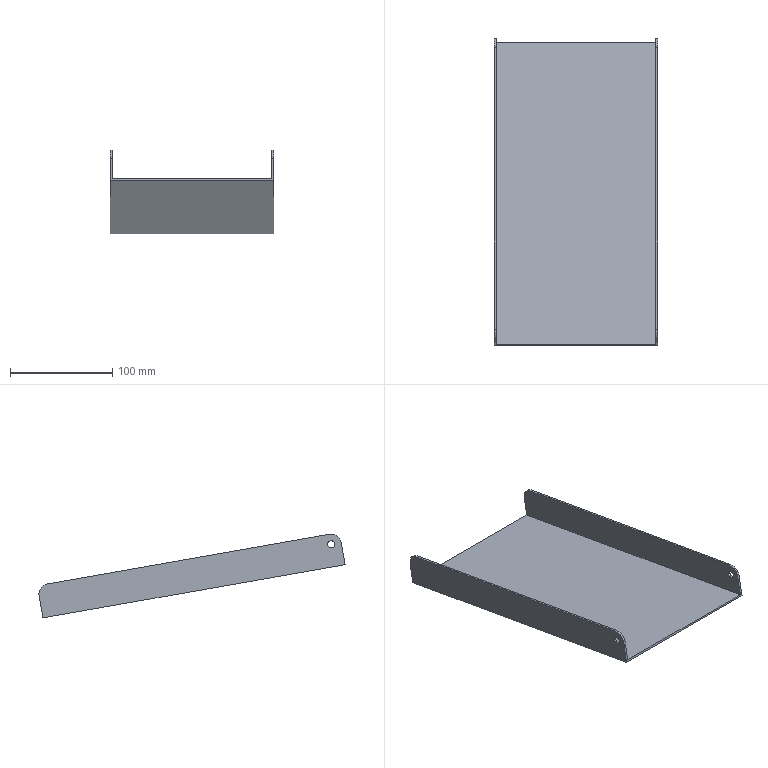Part | NX | features HB 2 | 1 solid | 16 faces | box 160 x 300.028 x 82.132 mm | volume 131949 mm3 | plane 10 | cylinder 6 | commonest cylinder face diameters 20 x4 7 x2
STEP:
#1=CARTESIAN_POINT('',(116.,686.06,-368.904));
#2=VERTEX_POINT('',#1);
#3=CARTESIAN_POINT('',(116.,686.966,-372.285));
#4=DIRECTION('',(-1.,0.,0.));
#5=DIRECTION('',(0.,-0.2588,0.9659));
#6=AXIS2_PLACEMENT_3D('',#3,#4,#5);
#7=CIRCLE('',#6,3.5);
#8=EDGE_CURVE('',#2,#2,#7,.T.);
#9=ORIENTED_EDGE('',*,*,#8,.T.);
#10=EDGE_LOOP('',(#9));
#11=FACE_BOUND('',#10,.T.);
#12=CARTESIAN_POINT('',(118.,686.06,-368.904));
#13=VERTEX_POINT('',#12);
#14=CARTESIAN_POINT('',(118.,686.966,-372.285));
#15=DIRECTION('',(1.,0.,0.));
#16=DIRECTION('',(0.,-0.2588,0.9659));
#17=AXIS2_PLACEMENT_3D('',#14,#15,#16);
#18=CIRCLE('',#17,3.5);
#19=EDGE_CURVE('',#13,#13,#18,.T.);
#20=ORIENTED_EDGE('',*,*,#19,.T.);
#21=EDGE_LOOP('',(#20));
#22=FACE_BOUND('',#21,.T.);
#23=CARTESIAN_POINT('',(826.,686.966,-372.285));
#24=DIRECTION('',(-1.,0.,0.));
#25=DIRECTION('',(0.,0.2588,-0.9659));
#26=AXIS2_PLACEMENT_3D('',#23,#24,#25);
#27=CYLINDRICAL_SURFACE('',#26,3.5);
#28=ADVANCED_FACE('',(#11,#22),#27,.F.);
#29=CARTESIAN_POINT('',(116.,688.702,-362.437));
#30=VERTEX_POINT('',#29);
#31=CARTESIAN_POINT('',(116.,965.062,-411.167));
#32=VERTEX_POINT('',#31);
#33=CARTESIAN_POINT('',(116.,564.245,-340.492));
#34=DIRECTION('',(0.,0.9848,-0.1736));
#35=VECTOR('',#34,1000.);
#36=LINE('',#33,#35);
#37=EDGE_CURVE('',#30,#32,#36,.T.);
#38=ORIENTED_EDGE('',*,*,#37,.F.);
#39=CARTESIAN_POINT('',(118.,688.702,-362.437));
#40=VERTEX_POINT('',#39);
#41=CARTESIAN_POINT('',(220.,688.702,-362.437));
#42=DIRECTION('',(1.,0.,0.));
#43=VECTOR('',#42,1000.);
#44=LINE('',#41,#43);
#45=EDGE_CURVE('',#30,#40,#44,.T.);
#46=ORIENTED_EDGE('',*,*,#45,.T.);
#47=CARTESIAN_POINT('',(118.,965.062,-411.167));
#48=VERTEX_POINT('',#47);
#49=CARTESIAN_POINT('',(118.,564.245,-340.492));
#50=DIRECTION('',(0.,0.9848,-0.1736));
#51=VECTOR('',#50,1000.);
#52=LINE('',#49,#51);
#53=EDGE_CURVE('',#40,#48,#52,.T.);
#54=ORIENTED_EDGE('',*,*,#53,.T.);
#55=CARTESIAN_POINT('',(220.,965.062,-411.167));
#56=DIRECTION('',(1.,0.,0.));
#57=VECTOR('',#56,1000.);
#58=LINE('',#55,#57);
#59=EDGE_CURVE('',#32,#48,#58,.T.);
#60=ORIENTED_EDGE('',*,*,#59,.F.);
#61=EDGE_LOOP('',(#38,#46,#54,#60));
#62=FACE_BOUND('',#61,.T.);
#63=CARTESIAN_POINT('',(220.,564.245,-340.492));
#64=DIRECTION('',(0.,-0.1736,-0.9848));
#65=DIRECTION('',(0.,0.9848,-0.1736));
#66=AXIS2_PLACEMENT_3D('',#63,#64,#65);
#67=PLANE('',#66);
#68=ADVANCED_FACE('',(#62),#67,.F.);
#69=CARTESIAN_POINT('',(116.,973.174,-422.751));
#70=VERTEX_POINT('',#69);
#71=CARTESIAN_POINT('',(116.,963.326,-421.015));
#72=DIRECTION('',(1.,0.,0.));
#73=DIRECTION('',(0.,-0.2588,0.9659));
#74=AXIS2_PLACEMENT_3D('',#71,#72,#73);
#75=CIRCLE('',#74,10.);
#76=EDGE_CURVE('',#70,#32,#75,.T.);
#77=ORIENTED_EDGE('',*,*,#76,.T.);
#78=ORIENTED_EDGE('',*,*,#59,.T.);
#79=CARTESIAN_POINT('',(118.,973.174,-422.751));
#80=VERTEX_POINT('',#79);
#81=CARTESIAN_POINT('',(118.,963.326,-421.015));
#82=DIRECTION('',(-1.,0.,0.));
#83=DIRECTION('',(0.,-0.2588,0.9659));
#84=AXIS2_PLACEMENT_3D('',#81,#82,#83);
#85=CIRCLE('',#84,10.);
#86=EDGE_CURVE('',#48,#80,#85,.T.);
#87=ORIENTED_EDGE('',*,*,#86,.T.);
#88=CARTESIAN_POINT('',(180.,973.174,-422.751));
#89=DIRECTION('',(-1.,0.,0.));
#90=VECTOR('',#89,1000.);
#91=LINE('',#88,#90);
#92=EDGE_CURVE('',#80,#70,#91,.T.);
#93=ORIENTED_EDGE('',*,*,#92,.T.);
#94=EDGE_LOOP('',(#77,#78,#87,#93));
#95=FACE_BOUND('',#94,.T.);
#96=CARTESIAN_POINT('',(220.,963.326,-421.015));
#97=DIRECTION('',(1.,0.,0.));
#98=DIRECTION('',(0.,-0.2588,0.9659));
#99=AXIS2_PLACEMENT_3D('',#96,#97,#98);
#100=CYLINDRICAL_SURFACE('',#99,10.);
#101=ADVANCED_FACE('',(#95),#100,.T.);
#102=ORIENTED_EDGE('',*,*,#53,.F.);
#103=CARTESIAN_POINT('',(118.,677.118,-370.549));
#104=VERTEX_POINT('',#103);
#105=CARTESIAN_POINT('',(118.,686.966,-372.285));
#106=DIRECTION('',(1.,0.,0.));
#107=DIRECTION('',(0.,0.5736,0.8192));
#108=AXIS2_PLACEMENT_3D('',#105,#106,#107);
#109=CIRCLE('',#108,10.);
#110=EDGE_CURVE('',#40,#104,#109,.T.);
#111=ORIENTED_EDGE('',*,*,#110,.T.);
#112=CARTESIAN_POINT('',(118.,673.298,-392.215));
#113=VERTEX_POINT('',#112);
#114=CARTESIAN_POINT('',(118.,673.645,-390.245));
#115=DIRECTION('',(0.,-0.1736,-0.9848));
#116=VECTOR('',#115,1000.);
#117=LINE('',#114,#116);
#118=EDGE_CURVE('',#104,#113,#117,.T.);
#119=ORIENTED_EDGE('',*,*,#118,.T.);
#120=CARTESIAN_POINT('',(118.,969.354,-444.417));
#121=VERTEX_POINT('',#120);
#122=CARTESIAN_POINT('',(118.,558.689,-372.006));
#123=DIRECTION('',(0.,-0.9848,0.1736));
#124=VECTOR('',#123,1000.);
#125=LINE('',#122,#124);
#126=EDGE_CURVE('',#121,#113,#125,.T.);
#127=ORIENTED_EDGE('',*,*,#126,.F.);
#128=CARTESIAN_POINT('',(118.,969.701,-442.448));
#129=DIRECTION('',(0.,-0.1736,-0.9848));
#130=VECTOR('',#129,1000.);
#131=LINE('',#128,#130);
#132=EDGE_CURVE('',#80,#121,#131,.T.);
#133=ORIENTED_EDGE('',*,*,#132,.F.);
#134=ORIENTED_EDGE('',*,*,#86,.F.);
#135=EDGE_LOOP('',(#102,#111,#119,#127,#133,#134));
#136=FACE_BOUND('',#135,.T.);
#137=ORIENTED_EDGE('',*,*,#19,.F.);
#138=EDGE_LOOP('',(#137));
#139=FACE_BOUND('',#138,.T.);
#140=CARTESIAN_POINT('',(118.,559.036,-370.036));
#141=DIRECTION('',(-1.,0.,0.));
#142=DIRECTION('',(0.,0.2588,-0.9659));
#143=AXIS2_PLACEMENT_3D('',#140,#141,#142);
#144=PLANE('',#143);
#145=ADVANCED_FACE('',(#136,#139),#144,.F.);
#146=CARTESIAN_POINT('',(116.,677.118,-370.549));
#147=VERTEX_POINT('',#146);
#148=CARTESIAN_POINT('',(116.,686.966,-372.285));
#149=DIRECTION('',(-1.,0.,0.));
#150=DIRECTION('',(0.,0.5736,0.8192));
#151=AXIS2_PLACEMENT_3D('',#148,#149,#150);
#152=CIRCLE('',#151,10.);
#153=EDGE_CURVE('',#147,#30,#152,.T.);
#154=ORIENTED_EDGE('',*,*,#153,.F.);
#155=CARTESIAN_POINT('',(220.,677.118,-370.549));
#156=DIRECTION('',(-1.,0.,0.));
#157=VECTOR('',#156,1000.);
#158=LINE('',#155,#157);
#159=EDGE_CURVE('',#104,#147,#158,.T.);
#160=ORIENTED_EDGE('',*,*,#159,.F.);
#161=ORIENTED_EDGE('',*,*,#110,.F.);
#162=ORIENTED_EDGE('',*,*,#45,.F.);
#163=EDGE_LOOP('',(#154,#160,#161,#162));
#164=FACE_BOUND('',#163,.T.);
#165=CARTESIAN_POINT('',(220.,686.966,-372.285));
#166=DIRECTION('',(1.,0.,0.));
#167=DIRECTION('',(0.,0.5736,0.8192));
#168=AXIS2_PLACEMENT_3D('',#165,#166,#167);
#169=CYLINDRICAL_SURFACE('',#168,10.);
#170=ADVANCED_FACE('',(#164),#169,.T.);
#171=ORIENTED_EDGE('',*,*,#76,.F.);
#172=CARTESIAN_POINT('',(116.,969.701,-442.448));
#173=VERTEX_POINT('',#172);
#174=CARTESIAN_POINT('',(116.,969.701,-442.448));
#175=DIRECTION('',(0.,-0.1736,-0.9848));
#176=VECTOR('',#175,1000.);
#177=LINE('',#174,#176);
#178=EDGE_CURVE('',#70,#173,#177,.T.);
#179=ORIENTED_EDGE('',*,*,#178,.T.);
#180=CARTESIAN_POINT('',(116.,673.645,-390.245));
#181=VERTEX_POINT('',#180);
#182=CARTESIAN_POINT('',(116.,559.036,-370.036));
#183=DIRECTION('',(0.,0.9848,-0.1736));
#184=VECTOR('',#183,1000.);
#185=LINE('',#182,#184);
#186=EDGE_CURVE('',#181,#173,#185,.T.);
#187=ORIENTED_EDGE('',*,*,#186,.F.);
#188=CARTESIAN_POINT('',(116.,673.645,-390.245));
#189=DIRECTION('',(0.,-0.1736,-0.9848));
#190=VECTOR('',#189,1000.);
#191=LINE('',#188,#190);
#192=EDGE_CURVE('',#147,#181,#191,.T.);
#193=ORIENTED_EDGE('',*,*,#192,.F.);
#194=ORIENTED_EDGE('',*,*,#153,.T.);
#195=ORIENTED_EDGE('',*,*,#37,.T.);
#196=EDGE_LOOP('',(#171,#179,#187,#193,#194,#195));
#197=FACE_BOUND('',#196,.T.);
#198=ORIENTED_EDGE('',*,*,#8,.F.);
#199=EDGE_LOOP('',(#198));
#200=FACE_BOUND('',#199,.T.);
#201=CARTESIAN_POINT('',(116.,559.036,-370.036));
#202=DIRECTION('',(-1.,0.,0.));
#203=DIRECTION('',(0.,-0.2588,0.9659));
#204=AXIS2_PLACEMENT_3D('',#201,#202,#203);
#205=PLANE('',#204);
#206=ADVANCED_FACE('',(#197,#200),#205,.T.);
#207=CARTESIAN_POINT('',(-40.,673.645,-390.245));
#208=VERTEX_POINT('',#207);
#209=CARTESIAN_POINT('',(180.,673.645,-390.245));
#210=DIRECTION('',(1.,0.,0.));
#211=VECTOR('',#210,1000.);
#212=LINE('',#209,#211);
#213=EDGE_CURVE('',#208,#181,#212,.T.);
#214=ORIENTED_EDGE('',*,*,#213,.F.);
#215=CARTESIAN_POINT('',(-40.,677.118,-370.549));
#216=VERTEX_POINT('',#215);
#217=CARTESIAN_POINT('',(-40.,673.645,-390.245));
#218=DIRECTION('',(0.,-0.1736,-0.9848));
#219=VECTOR('',#218,1000.);
#220=LINE('',#217,#219);
#221=EDGE_CURVE('',#216,#208,#220,.T.);
#222=ORIENTED_EDGE('',*,*,#221,.F.);
#223=CARTESIAN_POINT('',(-42.,677.118,-370.549));
#224=VERTEX_POINT('',#223);
#225=CARTESIAN_POINT('',(180.,677.118,-370.549));
#226=DIRECTION('',(-1.,0.,0.));
#227=VECTOR('',#226,1000.);
#228=LINE('',#225,#227);
#229=EDGE_CURVE('',#216,#224,#228,.T.);
#230=ORIENTED_EDGE('',*,*,#229,.T.);
#231=CARTESIAN_POINT('',(-42.,673.298,-392.215));
#232=VERTEX_POINT('',#231);
#233=CARTESIAN_POINT('',(-42.,673.645,-390.245));
#234=DIRECTION('',(0.,-0.1736,-0.9848));
#235=VECTOR('',#234,1000.);
#236=LINE('',#233,#235);
#237=EDGE_CURVE('',#224,#232,#236,.T.);
#238=ORIENTED_EDGE('',*,*,#237,.T.);
#239=CARTESIAN_POINT('',(180.,673.298,-392.215));
#240=DIRECTION('',(1.,0.,0.));
#241=VECTOR('',#240,1000.);
#242=LINE('',#239,#241);
#243=EDGE_CURVE('',#232,#113,#242,.T.);
#244=ORIENTED_EDGE('',*,*,#243,.T.);
#245=ORIENTED_EDGE('',*,*,#118,.F.);
#246=ORIENTED_EDGE('',*,*,#159,.T.);
#247=ORIENTED_EDGE('',*,*,#192,.T.);
#248=EDGE_LOOP('',(#214,#222,#230,#238,#244,#245,#246,#247));
#249=FACE_BOUND('',#248,.T.);
#250=CARTESIAN_POINT('',(180.,673.645,-390.245));
#251=DIRECTION('',(0.,0.9848,-0.1736));
#252=DIRECTION('',(0.,-0.1736,-0.9848));
#253=AXIS2_PLACEMENT_3D('',#250,#251,#252);
#254=PLANE('',#253);
#255=ADVANCED_FACE('',(#249),#254,.F.);
#256=ORIENTED_EDGE('',*,*,#178,.F.);
#257=ORIENTED_EDGE('',*,*,#92,.F.);
#258=ORIENTED_EDGE('',*,*,#132,.T.);
#259=CARTESIAN_POINT('',(-42.,969.354,-444.417));
#260=VERTEX_POINT('',#259);
#261=CARTESIAN_POINT('',(180.,969.354,-444.417));
#262=DIRECTION('',(1.,0.,0.));
#263=VECTOR('',#262,1000.);
#264=LINE('',#261,#263);
#265=EDGE_CURVE('',#260,#121,#264,.T.);
#266=ORIENTED_EDGE('',*,*,#265,.F.);
#267=CARTESIAN_POINT('',(-42.,973.174,-422.751));
#268=VERTEX_POINT('',#267);
#269=CARTESIAN_POINT('',(-42.,969.701,-442.448));
#270=DIRECTION('',(0.,-0.1736,-0.9848));
#271=VECTOR('',#270,1000.);
#272=LINE('',#269,#271);
#273=EDGE_CURVE('',#268,#260,#272,.T.);
#274=ORIENTED_EDGE('',*,*,#273,.F.);
#275=CARTESIAN_POINT('',(-40.,973.174,-422.751));
#276=VERTEX_POINT('',#275);
#277=CARTESIAN_POINT('',(263.,973.174,-422.751));
#278=DIRECTION('',(-1.,0.,0.));
#279=VECTOR('',#278,1000.);
#280=LINE('',#277,#279);
#281=EDGE_CURVE('',#276,#268,#280,.T.);
#282=ORIENTED_EDGE('',*,*,#281,.F.);
#283=CARTESIAN_POINT('',(-40.,969.701,-442.448));
#284=VERTEX_POINT('',#283);
#285=CARTESIAN_POINT('',(-40.,969.701,-442.448));
#286=DIRECTION('',(0.,-0.1736,-0.9848));
#287=VECTOR('',#286,1000.);
#288=LINE('',#285,#287);
#289=EDGE_CURVE('',#276,#284,#288,.T.);
#290=ORIENTED_EDGE('',*,*,#289,.T.);
#291=CARTESIAN_POINT('',(180.,969.701,-442.448));
#292=DIRECTION('',(1.,0.,0.));
#293=VECTOR('',#292,1000.);
#294=LINE('',#291,#293);
#295=EDGE_CURVE('',#284,#173,#294,.T.);
#296=ORIENTED_EDGE('',*,*,#295,.T.);
#297=EDGE_LOOP('',(#256,#257,#258,#266,#274,#282,#290,#296));
#298=FACE_BOUND('',#297,.T.);
#299=CARTESIAN_POINT('',(180.,969.701,-442.448));
#300=DIRECTION('',(0.,-0.9848,0.1736));
#301=DIRECTION('',(0.,-0.1736,-0.9848));
#302=AXIS2_PLACEMENT_3D('',#299,#300,#301);
#303=PLANE('',#302);
#304=ADVANCED_FACE('',(#298),#303,.F.);
#305=ORIENTED_EDGE('',*,*,#126,.T.);
#306=ORIENTED_EDGE('',*,*,#243,.F.);
#307=CARTESIAN_POINT('',(-42.,558.689,-372.006));
#308=DIRECTION('',(0.,0.9848,-0.1736));
#309=VECTOR('',#308,1000.);
#310=LINE('',#307,#309);
#311=EDGE_CURVE('',#232,#260,#310,.T.);
#312=ORIENTED_EDGE('',*,*,#311,.T.);
#313=ORIENTED_EDGE('',*,*,#265,.T.);
#314=EDGE_LOOP('',(#305,#306,#312,#313));
#315=FACE_BOUND('',#314,.T.);
#316=CARTESIAN_POINT('',(180.,558.689,-372.006));
#317=DIRECTION('',(0.,0.1736,0.9848));
#318=DIRECTION('',(-1.,0.,0.));
#319=AXIS2_PLACEMENT_3D('',#316,#317,#318);
#320=PLANE('',#319);
#321=ADVANCED_FACE('',(#315),#320,.F.);
#322=ORIENTED_EDGE('',*,*,#295,.F.);
#323=CARTESIAN_POINT('',(-40.,559.036,-370.036));
#324=DIRECTION('',(0.,-0.9848,0.1736));
#325=VECTOR('',#324,1000.);
#326=LINE('',#323,#325);
#327=EDGE_CURVE('',#284,#208,#326,.T.);
#328=ORIENTED_EDGE('',*,*,#327,.T.);
#329=ORIENTED_EDGE('',*,*,#213,.T.);
#330=ORIENTED_EDGE('',*,*,#186,.T.);
#331=EDGE_LOOP('',(#322,#328,#329,#330));
#332=FACE_BOUND('',#331,.T.);
#333=CARTESIAN_POINT('',(180.,559.036,-370.036));
#334=DIRECTION('',(0.,0.1736,0.9848));
#335=DIRECTION('',(-1.,0.,0.));
#336=AXIS2_PLACEMENT_3D('',#333,#334,#335);
#337=PLANE('',#336);
#338=ADVANCED_FACE('',(#332),#337,.T.);
#339=CARTESIAN_POINT('',(-42.,687.872,-375.666));
#340=VERTEX_POINT('',#339);
#341=CARTESIAN_POINT('',(-42.,686.966,-372.285));
#342=DIRECTION('',(-1.,0.,0.));
#343=DIRECTION('',(0.,0.2588,-0.9659));
#344=AXIS2_PLACEMENT_3D('',#341,#342,#343);
#345=CIRCLE('',#344,3.5);
#346=EDGE_CURVE('',#340,#340,#345,.T.);
#347=ORIENTED_EDGE('',*,*,#346,.F.);
#348=EDGE_LOOP('',(#347));
#349=FACE_BOUND('',#348,.T.);
#350=ORIENTED_EDGE('',*,*,#311,.F.);
#351=ORIENTED_EDGE('',*,*,#237,.F.);
#352=CARTESIAN_POINT('',(-42.,688.702,-362.437));
#353=VERTEX_POINT('',#352);
#354=CARTESIAN_POINT('',(-42.,686.966,-372.285));
#355=DIRECTION('',(-1.,0.,0.));
#356=DIRECTION('',(0.,-0.5736,-0.8192));
#357=AXIS2_PLACEMENT_3D('',#354,#355,#356);
#358=CIRCLE('',#357,10.);
#359=EDGE_CURVE('',#224,#353,#358,.T.);
#360=ORIENTED_EDGE('',*,*,#359,.T.);
#361=CARTESIAN_POINT('',(-42.,965.062,-411.167));
#362=VERTEX_POINT('',#361);
#363=CARTESIAN_POINT('',(-42.,564.245,-340.492));
#364=DIRECTION('',(0.,0.9848,-0.1736));
#365=VECTOR('',#364,1000.);
#366=LINE('',#363,#365);
#367=EDGE_CURVE('',#353,#362,#366,.T.);
#368=ORIENTED_EDGE('',*,*,#367,.T.);
#369=CARTESIAN_POINT('',(-42.,963.326,-421.015));
#370=DIRECTION('',(1.,0.,0.));
#371=DIRECTION('',(0.,0.2588,-0.9659));
#372=AXIS2_PLACEMENT_3D('',#369,#370,#371);
#373=CIRCLE('',#372,10.);
#374=EDGE_CURVE('',#268,#362,#373,.T.);
#375=ORIENTED_EDGE('',*,*,#374,.F.);
#376=ORIENTED_EDGE('',*,*,#273,.T.);
#377=EDGE_LOOP('',(#350,#351,#360,#368,#375,#376));
#378=FACE_BOUND('',#377,.T.);
#379=CARTESIAN_POINT('',(-42.,559.036,-370.036));
#380=DIRECTION('',(1.,0.,0.));
#381=DIRECTION('',(0.,-0.2588,0.9659));
#382=AXIS2_PLACEMENT_3D('',#379,#380,#381);
#383=PLANE('',#382);
#384=ADVANCED_FACE('',(#349,#378),#383,.F.);
#385=ORIENTED_EDGE('',*,*,#367,.F.);
#386=CARTESIAN_POINT('',(-40.,688.702,-362.437));
#387=VERTEX_POINT('',#386);
#388=CARTESIAN_POINT('',(5.,688.702,-362.437));
#389=DIRECTION('',(1.,0.,0.));
#390=VECTOR('',#389,1000.);
#391=LINE('',#388,#390);
#392=EDGE_CURVE('',#353,#387,#391,.T.);
#393=ORIENTED_EDGE('',*,*,#392,.T.);
#394=CARTESIAN_POINT('',(-40.,965.062,-411.167));
#395=VERTEX_POINT('',#394);
#396=CARTESIAN_POINT('',(-40.,564.245,-340.492));
#397=DIRECTION('',(0.,0.9848,-0.1736));
#398=VECTOR('',#397,1000.);
#399=LINE('',#396,#398);
#400=EDGE_CURVE('',#387,#395,#399,.T.);
#401=ORIENTED_EDGE('',*,*,#400,.T.);
#402=CARTESIAN_POINT('',(5.,965.062,-411.167));
#403=DIRECTION('',(1.,0.,0.));
#404=VECTOR('',#403,1000.);
#405=LINE('',#402,#404);
#406=EDGE_CURVE('',#362,#395,#405,.T.);
#407=ORIENTED_EDGE('',*,*,#406,.F.);
#408=EDGE_LOOP('',(#385,#393,#401,#407));
#409=FACE_BOUND('',#408,.T.);
#410=CARTESIAN_POINT('',(5.,564.245,-340.492));
#411=DIRECTION('',(0.,-0.1736,-0.9848));
#412=DIRECTION('',(0.,0.9848,-0.1736));
#413=AXIS2_PLACEMENT_3D('',#410,#411,#412);
#414=PLANE('',#413);
#415=ADVANCED_FACE('',(#409),#414,.F.);
#416=CARTESIAN_POINT('',(-40.,687.872,-375.666));
#417=VERTEX_POINT('',#416);
#418=CARTESIAN_POINT('',(-40.,686.966,-372.285));
#419=DIRECTION('',(-1.,0.,0.));
#420=DIRECTION('',(0.,0.2588,-0.9659));
#421=AXIS2_PLACEMENT_3D('',#418,#419,#420);
#422=CIRCLE('',#421,3.5);
#423=EDGE_CURVE('',#417,#417,#422,.T.);
#424=ORIENTED_EDGE('',*,*,#423,.T.);
#425=EDGE_LOOP('',(#424));
#426=FACE_BOUND('',#425,.T.);
#427=ORIENTED_EDGE('',*,*,#327,.F.);
#428=ORIENTED_EDGE('',*,*,#289,.F.);
#429=CARTESIAN_POINT('',(-40.,963.326,-421.015));
#430=DIRECTION('',(-1.,0.,0.));
#431=DIRECTION('',(0.,0.2588,-0.9659));
#432=AXIS2_PLACEMENT_3D('',#429,#430,#431);
#433=CIRCLE('',#432,10.);
#434=EDGE_CURVE('',#395,#276,#433,.T.);
#435=ORIENTED_EDGE('',*,*,#434,.F.);
#436=ORIENTED_EDGE('',*,*,#400,.F.);
#437=CARTESIAN_POINT('',(-40.,686.966,-372.285));
#438=DIRECTION('',(1.,0.,0.));
#439=DIRECTION('',(0.,-0.5736,-0.8192));
#440=AXIS2_PLACEMENT_3D('',#437,#438,#439);
#441=CIRCLE('',#440,10.);
#442=EDGE_CURVE('',#387,#216,#441,.T.);
#443=ORIENTED_EDGE('',*,*,#442,.T.);
#444=ORIENTED_EDGE('',*,*,#221,.T.);
#445=EDGE_LOOP('',(#427,#428,#435,#436,#443,#444));
#446=FACE_BOUND('',#445,.T.);
#447=CARTESIAN_POINT('',(-40.,559.036,-370.036));
#448=DIRECTION('',(1.,0.,0.));
#449=DIRECTION('',(0.,-0.2588,0.9659));
#450=AXIS2_PLACEMENT_3D('',#447,#448,#449);
#451=PLANE('',#450);
#452=ADVANCED_FACE('',(#426,#446),#451,.T.);
#453=ORIENTED_EDGE('',*,*,#434,.T.);
#454=ORIENTED_EDGE('',*,*,#281,.T.);
#455=ORIENTED_EDGE('',*,*,#374,.T.);
#456=ORIENTED_EDGE('',*,*,#406,.T.);
#457=EDGE_LOOP('',(#453,#454,#455,#456));
#458=FACE_BOUND('',#457,.T.);
#459=CARTESIAN_POINT('',(263.,963.326,-421.015));
#460=DIRECTION('',(-1.,0.,0.));
#461=DIRECTION('',(0.,0.2588,-0.9659));
#462=AXIS2_PLACEMENT_3D('',#459,#460,#461);
#463=CYLINDRICAL_SURFACE('',#462,10.);
#464=ADVANCED_FACE('',(#458),#463,.T.);
#465=ORIENTED_EDGE('',*,*,#442,.F.);
#466=ORIENTED_EDGE('',*,*,#392,.F.);
#467=ORIENTED_EDGE('',*,*,#359,.F.);
#468=ORIENTED_EDGE('',*,*,#229,.F.);
#469=EDGE_LOOP('',(#465,#466,#467,#468));
#470=FACE_BOUND('',#469,.T.);
#471=CARTESIAN_POINT('',(263.,686.966,-372.285));
#472=DIRECTION('',(-1.,0.,0.));
#473=DIRECTION('',(0.,-0.5736,-0.8192));
#474=AXIS2_PLACEMENT_3D('',#471,#472,#473);
#475=CYLINDRICAL_SURFACE('',#474,10.);
#476=ADVANCED_FACE('',(#470),#475,.T.);
#477=ORIENTED_EDGE('',*,*,#423,.F.);
#478=EDGE_LOOP('',(#477));
#479=FACE_BOUND('',#478,.T.);
#480=ORIENTED_EDGE('',*,*,#346,.T.);
#481=EDGE_LOOP('',(#480));
#482=FACE_BOUND('',#481,.T.);
#483=CARTESIAN_POINT('',(3.,686.966,-372.285));
#484=DIRECTION('',(1.,0.,0.));
#485=DIRECTION('',(0.,-0.2588,0.9659));
#486=AXIS2_PLACEMENT_3D('',#483,#484,#485);
#487=CYLINDRICAL_SURFACE('',#486,3.5);
#488=ADVANCED_FACE('',(#479,#482),#487,.F.);
#489=CLOSED_SHELL('',(#28,#68,#101,#145,#170,#206,#255,#304,#321,#338,#384,#415,#452,#464,#476,#488));
#490=MANIFOLD_SOLID_BREP('',#489);
#491=(LENGTH_UNIT()NAMED_UNIT(*)SI_UNIT(.MILLI.,.METRE.));
#492=UNCERTAINTY_MEASURE_WITH_UNIT(LENGTH_MEASURE(0.00001),#491,'','');
#493=(NAMED_UNIT(*)PLANE_ANGLE_UNIT()SI_UNIT($,.RADIAN.));
#494=(NAMED_UNIT(*)SI_UNIT($,.STERADIAN.)SOLID_ANGLE_UNIT());
#495=(GEOMETRIC_REPRESENTATION_CONTEXT(3)GLOBAL_UNCERTAINTY_ASSIGNED_CONTEXT((#492))GLOBAL_UNIT_ASSIGNED_CONTEXT((#491,#493,#494))REPRESENTATION_CONTEXT('',''));
#496=ADVANCED_BREP_SHAPE_REPRESENTATION('',(#490),#495);